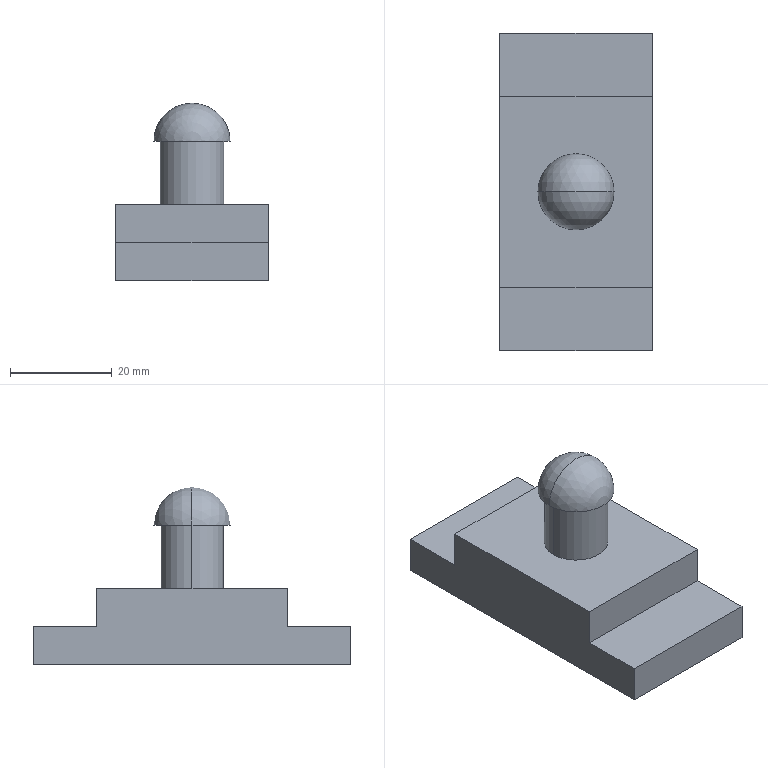Part | SolidWorks | features ICE 2, Extrusion 1, Revolution 1, Scale 1 | 1 solid | 15 faces | box 30 x 62.5 x 35 mm | volume 24918 mm3 | plane 11 | sphere 2 | cylinder 2 | commonest cylinder face diameters 12.5 x2
STEP:
#1=CARTESIAN_POINT('',(0.,0.,35.));
#2=VERTEX_POINT('',#1);
#3=CARTESIAN_POINT('',(7.5,0.,27.5));
#4=VERTEX_POINT('',#3);
#5=CARTESIAN_POINT('',(0.,0.,27.5));
#6=DIRECTION('',(0.,1.,0.));
#7=DIRECTION('',(0.,0.,1.));
#8=AXIS2_PLACEMENT_3D('',#5,#6,#7);
#9=CIRCLE('',#8,7.5);
#10=EDGE_CURVE('',#2,#4,#9,.T.);
#11=ORIENTED_EDGE('',*,*,#10,.F.);
#12=CARTESIAN_POINT('',(-7.5,0.,27.5));
#13=VERTEX_POINT('',#12);
#14=CARTESIAN_POINT('',(0.,0.,27.5));
#15=DIRECTION('',(0.,-1.,0.));
#16=DIRECTION('',(1.,0.,0.));
#17=AXIS2_PLACEMENT_3D('',#14,#15,#16);
#18=CIRCLE('',#17,7.5);
#19=EDGE_CURVE('',#2,#13,#18,.T.);
#20=ORIENTED_EDGE('',*,*,#19,.T.);
#21=CARTESIAN_POINT('',(0.,0.,27.5));
#22=DIRECTION('',(0.,0.,-1.));
#23=DIRECTION('',(-1.,0.,0.));
#24=AXIS2_PLACEMENT_3D('',#21,#22,#23);
#25=CIRCLE('',#24,7.5);
#26=EDGE_CURVE('',#4,#13,#25,.T.);
#27=ORIENTED_EDGE('',*,*,#26,.F.);
#28=EDGE_LOOP('',(#11,#20,#27));
#29=FACE_OUTER_BOUND('',#28,.T.);
#30=CARTESIAN_POINT('',(0.,0.,27.5));
#31=DIRECTION('',(0.,-1.,0.));
#32=DIRECTION('',(1.,0.,0.));
#33=AXIS2_PLACEMENT_3D('',#30,#31,#32);
#34=SPHERICAL_SURFACE('',#33,7.5);
#35=ADVANCED_FACE('',(#29),#34,.T.);
#36=CARTESIAN_POINT('',(6.25,0.,27.5));
#37=VERTEX_POINT('',#36);
#38=CARTESIAN_POINT('',(-6.25,0.,27.5));
#39=VERTEX_POINT('',#38);
#40=CARTESIAN_POINT('',(0.,0.,27.5));
#41=DIRECTION('',(0.,0.,1.));
#42=DIRECTION('',(1.,0.,0.));
#43=AXIS2_PLACEMENT_3D('',#40,#41,#42);
#44=CIRCLE('',#43,6.25);
#45=EDGE_CURVE('',#37,#39,#44,.T.);
#46=ORIENTED_EDGE('',*,*,#45,.F.);
#47=CARTESIAN_POINT('',(6.25,0.,15.));
#48=VERTEX_POINT('',#47);
#49=CARTESIAN_POINT('',(6.25,0.,27.5));
#50=DIRECTION('',(0.,0.,-1.));
#51=VECTOR('',#50,1000.);
#52=LINE('',#49,#51);
#53=EDGE_CURVE('',#37,#48,#52,.T.);
#54=ORIENTED_EDGE('',*,*,#53,.T.);
#55=CARTESIAN_POINT('',(-6.25,0.,15.));
#56=VERTEX_POINT('',#55);
#57=CARTESIAN_POINT('',(0.,0.,15.));
#58=DIRECTION('',(0.,0.,1.));
#59=DIRECTION('',(1.,0.,0.));
#60=AXIS2_PLACEMENT_3D('',#57,#58,#59);
#61=CIRCLE('',#60,6.25);
#62=EDGE_CURVE('',#48,#56,#61,.T.);
#63=ORIENTED_EDGE('',*,*,#62,.T.);
#64=CARTESIAN_POINT('',(-6.25,0.,27.5));
#65=DIRECTION('',(0.,0.,-1.));
#66=VECTOR('',#65,1000.);
#67=LINE('',#64,#66);
#68=EDGE_CURVE('',#39,#56,#67,.T.);
#69=ORIENTED_EDGE('',*,*,#68,.F.);
#70=EDGE_LOOP('',(#46,#54,#63,#69));
#71=FACE_OUTER_BOUND('',#70,.T.);
#72=CARTESIAN_POINT('',(0.,0.,27.5));
#73=DIRECTION('',(0.,0.,-1.));
#74=DIRECTION('',(-1.,0.,0.));
#75=AXIS2_PLACEMENT_3D('',#72,#73,#74);
#76=CYLINDRICAL_SURFACE('',#75,6.25);
#77=ADVANCED_FACE('',(#71),#76,.T.);
#78=CARTESIAN_POINT('',(-15.,-18.75,7.5));
#79=VERTEX_POINT('',#78);
#80=CARTESIAN_POINT('',(15.,-18.75,7.5));
#81=VERTEX_POINT('',#80);
#82=CARTESIAN_POINT('',(-15.,-18.75,7.5));
#83=DIRECTION('',(1.,0.,0.));
#84=VECTOR('',#83,1000.);
#85=LINE('',#82,#84);
#86=EDGE_CURVE('',#79,#81,#85,.T.);
#87=ORIENTED_EDGE('',*,*,#86,.F.);
#88=CARTESIAN_POINT('',(-15.,-31.25,7.5));
#89=VERTEX_POINT('',#88);
#90=CARTESIAN_POINT('',(-15.,31.25,7.5));
#91=DIRECTION('',(0.,-1.,0.));
#92=VECTOR('',#91,1000.);
#93=LINE('',#90,#92);
#94=EDGE_CURVE('',#79,#89,#93,.T.);
#95=ORIENTED_EDGE('',*,*,#94,.T.);
#96=CARTESIAN_POINT('',(15.,-31.25,7.5));
#97=VERTEX_POINT('',#96);
#98=CARTESIAN_POINT('',(-15.,-31.25,7.5));
#99=DIRECTION('',(1.,0.,0.));
#100=VECTOR('',#99,1000.);
#101=LINE('',#98,#100);
#102=EDGE_CURVE('',#89,#97,#101,.T.);
#103=ORIENTED_EDGE('',*,*,#102,.T.);
#104=CARTESIAN_POINT('',(15.,31.25,7.5));
#105=DIRECTION('',(0.,1.,0.));
#106=VECTOR('',#105,1000.);
#107=LINE('',#104,#106);
#108=EDGE_CURVE('',#97,#81,#107,.T.);
#109=ORIENTED_EDGE('',*,*,#108,.T.);
#110=EDGE_LOOP('',(#87,#95,#103,#109));
#111=FACE_OUTER_BOUND('',#110,.T.);
#112=CARTESIAN_POINT('',(0.,0.,7.5));
#113=DIRECTION('',(0.,0.,1.));
#114=DIRECTION('',(1.,0.,0.));
#115=AXIS2_PLACEMENT_3D('',#112,#113,#114);
#116=PLANE('',#115);
#117=ADVANCED_FACE('',(#111),#116,.T.);
#118=CARTESIAN_POINT('',(15.,-31.25,0.));
#119=VERTEX_POINT('',#118);
#120=CARTESIAN_POINT('',(15.,31.25,0.));
#121=VERTEX_POINT('',#120);
#122=CARTESIAN_POINT('',(15.,31.25,0.));
#123=DIRECTION('',(0.,1.,0.));
#124=VECTOR('',#123,1000.);
#125=LINE('',#122,#124);
#126=EDGE_CURVE('',#119,#121,#125,.T.);
#127=ORIENTED_EDGE('',*,*,#126,.T.);
#128=CARTESIAN_POINT('',(15.,31.25,7.5));
#129=VERTEX_POINT('',#128);
#130=CARTESIAN_POINT('',(15.,31.25,7.5));
#131=DIRECTION('',(0.,0.,-1.));
#132=VECTOR('',#131,1000.);
#133=LINE('',#130,#132);
#134=EDGE_CURVE('',#129,#121,#133,.T.);
#135=ORIENTED_EDGE('',*,*,#134,.F.);
#136=CARTESIAN_POINT('',(15.,18.75,7.5));
#137=VERTEX_POINT('',#136);
#138=CARTESIAN_POINT('',(15.,31.25,7.5));
#139=DIRECTION('',(0.,1.,0.));
#140=VECTOR('',#139,1000.);
#141=LINE('',#138,#140);
#142=EDGE_CURVE('',#137,#129,#141,.T.);
#143=ORIENTED_EDGE('',*,*,#142,.F.);
#144=CARTESIAN_POINT('',(15.,18.75,15.));
#145=VERTEX_POINT('',#144);
#146=CARTESIAN_POINT('',(15.,18.75,15.));
#147=DIRECTION('',(0.,0.,-1.));
#148=VECTOR('',#147,1000.);
#149=LINE('',#146,#148);
#150=EDGE_CURVE('',#145,#137,#149,.T.);
#151=ORIENTED_EDGE('',*,*,#150,.F.);
#152=CARTESIAN_POINT('',(15.,-18.75,15.));
#153=VERTEX_POINT('',#152);
#154=CARTESIAN_POINT('',(15.,-18.75,15.));
#155=DIRECTION('',(0.,1.,0.));
#156=VECTOR('',#155,1000.);
#157=LINE('',#154,#156);
#158=EDGE_CURVE('',#153,#145,#157,.T.);
#159=ORIENTED_EDGE('',*,*,#158,.F.);
#160=CARTESIAN_POINT('',(15.,-18.75,15.));
#161=DIRECTION('',(0.,0.,-1.));
#162=VECTOR('',#161,1000.);
#163=LINE('',#160,#162);
#164=EDGE_CURVE('',#153,#81,#163,.T.);
#165=ORIENTED_EDGE('',*,*,#164,.T.);
#166=ORIENTED_EDGE('',*,*,#108,.F.);
#167=CARTESIAN_POINT('',(15.,-31.25,7.5));
#168=DIRECTION('',(0.,0.,-1.));
#169=VECTOR('',#168,1000.);
#170=LINE('',#167,#169);
#171=EDGE_CURVE('',#97,#119,#170,.T.);
#172=ORIENTED_EDGE('',*,*,#171,.T.);
#173=EDGE_LOOP('',(#127,#135,#143,#151,#159,#165,#166,#172));
#174=FACE_OUTER_BOUND('',#173,.T.);
#175=CARTESIAN_POINT('',(15.,31.25,7.5));
#176=DIRECTION('',(-1.,0.,0.));
#177=DIRECTION('',(0.,-1.,0.));
#178=AXIS2_PLACEMENT_3D('',#175,#176,#177);
#179=PLANE('',#178);
#180=ADVANCED_FACE('',(#174),#179,.F.);
#181=CARTESIAN_POINT('',(-15.,31.25,0.));
#182=VERTEX_POINT('',#181);
#183=CARTESIAN_POINT('',(-15.,31.25,0.));
#184=DIRECTION('',(-1.,0.,0.));
#185=VECTOR('',#184,1000.);
#186=LINE('',#183,#185);
#187=EDGE_CURVE('',#121,#182,#186,.T.);
#188=ORIENTED_EDGE('',*,*,#187,.T.);
#189=CARTESIAN_POINT('',(-15.,31.25,7.5));
#190=VERTEX_POINT('',#189);
#191=CARTESIAN_POINT('',(-15.,31.25,7.5));
#192=DIRECTION('',(0.,0.,-1.));
#193=VECTOR('',#192,1000.);
#194=LINE('',#191,#193);
#195=EDGE_CURVE('',#190,#182,#194,.T.);
#196=ORIENTED_EDGE('',*,*,#195,.F.);
#197=CARTESIAN_POINT('',(-15.,31.25,7.5));
#198=DIRECTION('',(-1.,0.,0.));
#199=VECTOR('',#198,1000.);
#200=LINE('',#197,#199);
#201=EDGE_CURVE('',#129,#190,#200,.T.);
#202=ORIENTED_EDGE('',*,*,#201,.F.);
#203=ORIENTED_EDGE('',*,*,#134,.T.);
#204=EDGE_LOOP('',(#188,#196,#202,#203));
#205=FACE_OUTER_BOUND('',#204,.T.);
#206=CARTESIAN_POINT('',(-15.,31.25,7.5));
#207=DIRECTION('',(0.,-1.,0.));
#208=DIRECTION('',(0.,0.,-1.));
#209=AXIS2_PLACEMENT_3D('',#206,#207,#208);
#210=PLANE('',#209);
#211=ADVANCED_FACE('',(#205),#210,.F.);
#212=CARTESIAN_POINT('',(-15.,-31.25,0.));
#213=VERTEX_POINT('',#212);
#214=CARTESIAN_POINT('',(-15.,31.25,0.));
#215=DIRECTION('',(0.,-1.,0.));
#216=VECTOR('',#215,1000.);
#217=LINE('',#214,#216);
#218=EDGE_CURVE('',#182,#213,#217,.T.);
#219=ORIENTED_EDGE('',*,*,#218,.T.);
#220=CARTESIAN_POINT('',(-15.,-31.25,7.5));
#221=DIRECTION('',(0.,0.,-1.));
#222=VECTOR('',#221,1000.);
#223=LINE('',#220,#222);
#224=EDGE_CURVE('',#89,#213,#223,.T.);
#225=ORIENTED_EDGE('',*,*,#224,.F.);
#226=ORIENTED_EDGE('',*,*,#94,.F.);
#227=CARTESIAN_POINT('',(-15.,-18.75,15.));
#228=VERTEX_POINT('',#227);
#229=CARTESIAN_POINT('',(-15.,-18.75,15.));
#230=DIRECTION('',(0.,0.,-1.));
#231=VECTOR('',#230,1000.);
#232=LINE('',#229,#231);
#233=EDGE_CURVE('',#228,#79,#232,.T.);
#234=ORIENTED_EDGE('',*,*,#233,.F.);
#235=CARTESIAN_POINT('',(-15.,18.75,15.));
#236=VERTEX_POINT('',#235);
#237=CARTESIAN_POINT('',(-15.,-18.75,15.));
#238=DIRECTION('',(0.,-1.,0.));
#239=VECTOR('',#238,1000.);
#240=LINE('',#237,#239);
#241=EDGE_CURVE('',#236,#228,#240,.T.);
#242=ORIENTED_EDGE('',*,*,#241,.F.);
#243=CARTESIAN_POINT('',(-15.,18.75,7.5));
#244=VERTEX_POINT('',#243);
#245=CARTESIAN_POINT('',(-15.,18.75,15.));
#246=DIRECTION('',(0.,0.,-1.));
#247=VECTOR('',#246,1000.);
#248=LINE('',#245,#247);
#249=EDGE_CURVE('',#236,#244,#248,.T.);
#250=ORIENTED_EDGE('',*,*,#249,.T.);
#251=CARTESIAN_POINT('',(-15.,31.25,7.5));
#252=DIRECTION('',(0.,-1.,0.));
#253=VECTOR('',#252,1000.);
#254=LINE('',#251,#253);
#255=EDGE_CURVE('',#190,#244,#254,.T.);
#256=ORIENTED_EDGE('',*,*,#255,.F.);
#257=ORIENTED_EDGE('',*,*,#195,.T.);
#258=EDGE_LOOP('',(#219,#225,#226,#234,#242,#250,#256,#257));
#259=FACE_OUTER_BOUND('',#258,.T.);
#260=CARTESIAN_POINT('',(-15.,31.25,7.5));
#261=DIRECTION('',(1.,0.,0.));
#262=DIRECTION('',(0.,1.,0.));
#263=AXIS2_PLACEMENT_3D('',#260,#261,#262);
#264=PLANE('',#263);
#265=ADVANCED_FACE('',(#259),#264,.F.);
#266=CARTESIAN_POINT('',(-15.,-31.25,0.));
#267=DIRECTION('',(1.,0.,0.));
#268=VECTOR('',#267,1000.);
#269=LINE('',#266,#268);
#270=EDGE_CURVE('',#213,#119,#269,.T.);
#271=ORIENTED_EDGE('',*,*,#270,.T.);
#272=ORIENTED_EDGE('',*,*,#171,.F.);
#273=ORIENTED_EDGE('',*,*,#102,.F.);
#274=ORIENTED_EDGE('',*,*,#224,.T.);
#275=EDGE_LOOP('',(#271,#272,#273,#274));
#276=FACE_OUTER_BOUND('',#275,.T.);
#277=CARTESIAN_POINT('',(-15.,-31.25,7.5));
#278=DIRECTION('',(0.,1.,0.));
#279=DIRECTION('',(0.,0.,1.));
#280=AXIS2_PLACEMENT_3D('',#277,#278,#279);
#281=PLANE('',#280);
#282=ADVANCED_FACE('',(#276),#281,.F.);
#283=CARTESIAN_POINT('',(-15.,18.75,7.5));
#284=DIRECTION('',(-1.,0.,0.));
#285=VECTOR('',#284,1000.);
#286=LINE('',#283,#285);
#287=EDGE_CURVE('',#137,#244,#286,.T.);
#288=ORIENTED_EDGE('',*,*,#287,.F.);
#289=ORIENTED_EDGE('',*,*,#142,.T.);
#290=ORIENTED_EDGE('',*,*,#201,.T.);
#291=ORIENTED_EDGE('',*,*,#255,.T.);
#292=EDGE_LOOP('',(#288,#289,#290,#291));
#293=FACE_OUTER_BOUND('',#292,.T.);
#294=CARTESIAN_POINT('',(0.,0.,7.5));
#295=DIRECTION('',(0.,0.,1.));
#296=DIRECTION('',(1.,0.,0.));
#297=AXIS2_PLACEMENT_3D('',#294,#295,#296);
#298=PLANE('',#297);
#299=ADVANCED_FACE('',(#293),#298,.T.);
#300=ORIENTED_EDGE('',*,*,#126,.F.);
#301=ORIENTED_EDGE('',*,*,#270,.F.);
#302=ORIENTED_EDGE('',*,*,#218,.F.);
#303=ORIENTED_EDGE('',*,*,#187,.F.);
#304=EDGE_LOOP('',(#300,#301,#302,#303));
#305=FACE_OUTER_BOUND('',#304,.T.);
#306=CARTESIAN_POINT('',(0.,0.,0.));
#307=DIRECTION('',(0.,0.,1.));
#308=DIRECTION('',(1.,0.,0.));
#309=AXIS2_PLACEMENT_3D('',#306,#307,#308);
#310=PLANE('',#309);
#311=ADVANCED_FACE('',(#305),#310,.F.);
#312=ORIENTED_EDGE('',*,*,#287,.T.);
#313=ORIENTED_EDGE('',*,*,#249,.F.);
#314=CARTESIAN_POINT('',(-15.,18.75,15.));
#315=DIRECTION('',(-1.,0.,0.));
#316=VECTOR('',#315,1000.);
#317=LINE('',#314,#316);
#318=EDGE_CURVE('',#145,#236,#317,.T.);
#319=ORIENTED_EDGE('',*,*,#318,.F.);
#320=ORIENTED_EDGE('',*,*,#150,.T.);
#321=EDGE_LOOP('',(#312,#313,#319,#320));
#322=FACE_OUTER_BOUND('',#321,.T.);
#323=CARTESIAN_POINT('',(-15.,18.75,15.));
#324=DIRECTION('',(0.,-1.,0.));
#325=DIRECTION('',(0.,0.,-1.));
#326=AXIS2_PLACEMENT_3D('',#323,#324,#325);
#327=PLANE('',#326);
#328=ADVANCED_FACE('',(#322),#327,.F.);
#329=ORIENTED_EDGE('',*,*,#86,.T.);
#330=ORIENTED_EDGE('',*,*,#164,.F.);
#331=CARTESIAN_POINT('',(-15.,-18.75,15.));
#332=DIRECTION('',(1.,0.,0.));
#333=VECTOR('',#332,1000.);
#334=LINE('',#331,#333);
#335=EDGE_CURVE('',#228,#153,#334,.T.);
#336=ORIENTED_EDGE('',*,*,#335,.F.);
#337=ORIENTED_EDGE('',*,*,#233,.T.);
#338=EDGE_LOOP('',(#329,#330,#336,#337));
#339=FACE_OUTER_BOUND('',#338,.T.);
#340=CARTESIAN_POINT('',(-15.,-18.75,15.));
#341=DIRECTION('',(0.,1.,0.));
#342=DIRECTION('',(0.,0.,1.));
#343=AXIS2_PLACEMENT_3D('',#340,#341,#342);
#344=PLANE('',#343);
#345=ADVANCED_FACE('',(#339),#344,.F.);
#346=CARTESIAN_POINT('',(0.,0.,15.));
#347=DIRECTION('',(0.,0.,1.));
#348=DIRECTION('',(1.,0.,0.));
#349=AXIS2_PLACEMENT_3D('',#346,#347,#348);
#350=CIRCLE('',#349,6.25);
#351=EDGE_CURVE('',#56,#48,#350,.T.);
#352=ORIENTED_EDGE('',*,*,#351,.F.);
#353=ORIENTED_EDGE('',*,*,#62,.F.);
#354=EDGE_LOOP('',(#352,#353));
#355=FACE_BOUND('',#354,.T.);
#356=ORIENTED_EDGE('',*,*,#158,.T.);
#357=ORIENTED_EDGE('',*,*,#318,.T.);
#358=ORIENTED_EDGE('',*,*,#241,.T.);
#359=ORIENTED_EDGE('',*,*,#335,.T.);
#360=EDGE_LOOP('',(#356,#357,#358,#359));
#361=FACE_OUTER_BOUND('',#360,.T.);
#362=CARTESIAN_POINT('',(0.,0.,15.));
#363=DIRECTION('',(0.,0.,-1.));
#364=DIRECTION('',(-1.,0.,0.));
#365=AXIS2_PLACEMENT_3D('',#362,#363,#364);
#366=PLANE('',#365);
#367=ADVANCED_FACE('',(#355,#361),#366,.F.);
#368=ORIENTED_EDGE('',*,*,#53,.F.);
#369=CARTESIAN_POINT('',(0.,0.,27.5));
#370=DIRECTION('',(0.,0.,1.));
#371=DIRECTION('',(1.,0.,0.));
#372=AXIS2_PLACEMENT_3D('',#369,#370,#371);
#373=CIRCLE('',#372,6.25);
#374=EDGE_CURVE('',#39,#37,#373,.T.);
#375=ORIENTED_EDGE('',*,*,#374,.F.);
#376=ORIENTED_EDGE('',*,*,#68,.T.);
#377=ORIENTED_EDGE('',*,*,#351,.T.);
#378=EDGE_LOOP('',(#368,#375,#376,#377));
#379=FACE_OUTER_BOUND('',#378,.T.);
#380=CARTESIAN_POINT('',(0.,0.,27.5));
#381=DIRECTION('',(0.,0.,-1.));
#382=DIRECTION('',(-1.,0.,0.));
#383=AXIS2_PLACEMENT_3D('',#380,#381,#382);
#384=CYLINDRICAL_SURFACE('',#383,6.25);
#385=ADVANCED_FACE('',(#379),#384,.T.);
#386=ORIENTED_EDGE('',*,*,#374,.T.);
#387=ORIENTED_EDGE('',*,*,#45,.T.);
#388=EDGE_LOOP('',(#386,#387));
#389=FACE_BOUND('',#388,.T.);
#390=ORIENTED_EDGE('',*,*,#26,.T.);
#391=CARTESIAN_POINT('',(0.,0.,27.5));
#392=DIRECTION('',(0.,0.,-1.));
#393=DIRECTION('',(-1.,0.,0.));
#394=AXIS2_PLACEMENT_3D('',#391,#392,#393);
#395=CIRCLE('',#394,7.5);
#396=EDGE_CURVE('',#13,#4,#395,.T.);
#397=ORIENTED_EDGE('',*,*,#396,.T.);
#398=EDGE_LOOP('',(#390,#397));
#399=FACE_OUTER_BOUND('',#398,.T.);
#400=CARTESIAN_POINT('',(0.,0.,27.5));
#401=DIRECTION('',(0.,0.,1.));
#402=DIRECTION('',(1.,0.,0.));
#403=AXIS2_PLACEMENT_3D('',#400,#401,#402);
#404=PLANE('',#403);
#405=ADVANCED_FACE('',(#389,#399),#404,.F.);
#406=ORIENTED_EDGE('',*,*,#19,.F.);
#407=ORIENTED_EDGE('',*,*,#10,.T.);
#408=ORIENTED_EDGE('',*,*,#396,.F.);
#409=EDGE_LOOP('',(#406,#407,#408));
#410=FACE_OUTER_BOUND('',#409,.T.);
#411=CARTESIAN_POINT('',(0.,0.,27.5));
#412=DIRECTION('',(0.,-1.,0.));
#413=DIRECTION('',(1.,0.,0.));
#414=AXIS2_PLACEMENT_3D('',#411,#412,#413);
#415=SPHERICAL_SURFACE('',#414,7.5);
#416=ADVANCED_FACE('',(#410),#415,.T.);
#417=CLOSED_SHELL('',(#35,#77,#117,#180,#211,#265,#282,#299,#311,#328,#345,#367,#385,#405,#416));
#418=MANIFOLD_SOLID_BREP('',#417);
#419=CARTESIAN_POINT('',(0.,0.,0.));
#420=DIRECTION('',(0.,0.,1.));
#421=DIRECTION('',(1.,0.,0.));
#422=AXIS2_PLACEMENT_3D('',#419,#420,#421);
#423=(LENGTH_UNIT()NAMED_UNIT(*)SI_UNIT(.MILLI.,.METRE.));
#424=UNCERTAINTY_MEASURE_WITH_UNIT(LENGTH_MEASURE(0.00001),#423,'','');
#425=(NAMED_UNIT(*)PLANE_ANGLE_UNIT()SI_UNIT($,.RADIAN.));
#426=(NAMED_UNIT(*)SI_UNIT($,.STERADIAN.)SOLID_ANGLE_UNIT());
#427=(GEOMETRIC_REPRESENTATION_CONTEXT(3)GLOBAL_UNCERTAINTY_ASSIGNED_CONTEXT((#424))GLOBAL_UNIT_ASSIGNED_CONTEXT((#423,#425,#426))REPRESENTATION_CONTEXT('',''));
#428=ADVANCED_BREP_SHAPE_REPRESENTATION('',(#418,#422),#427);